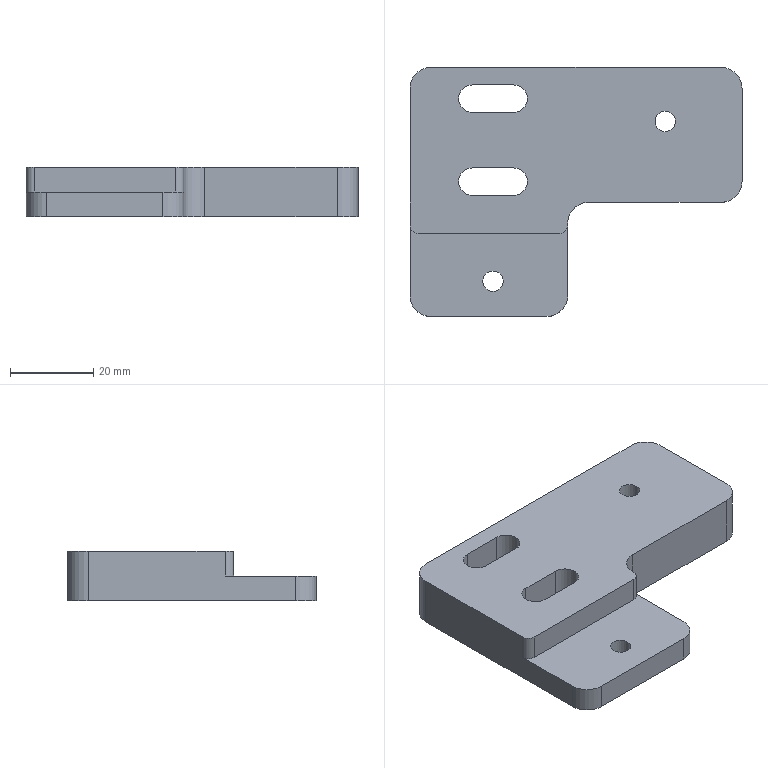Part | NX | 1 solid | 28 faces | box 80 x 60 x 12 mm | volume 36230 mm3 | cylinder 14 | plane 14 | commonest cylinder face diameters 10 x6 6.6 x4 4 x2 4.917 x2
STEP:
#1=CARTESIAN_POINT('',(-38.,-14.,6.));
#2=VERTEX_POINT('',#1);
#3=CARTESIAN_POINT('',(-40.,-12.,6.));
#4=VERTEX_POINT('',#3);
#5=CARTESIAN_POINT('',(-38.,-12.,6.));
#6=DIRECTION('',(0.,0.,-1.));
#7=DIRECTION('',(-0.7071,-0.7071,0.));
#8=AXIS2_PLACEMENT_3D('',#5,#6,#7);
#9=CIRCLE('',#8,2.);
#10=EDGE_CURVE('',#2,#4,#9,.T.);
#11=ORIENTED_EDGE('',*,*,#10,.T.);
#12=CARTESIAN_POINT('',(-40.,-12.,0.));
#13=VERTEX_POINT('',#12);
#14=CARTESIAN_POINT('',(-40.,-12.,0.));
#15=DIRECTION('',(0.,0.,-1.));
#16=VECTOR('',#15,1000.);
#17=LINE('',#14,#16);
#18=EDGE_CURVE('',#4,#13,#17,.T.);
#19=ORIENTED_EDGE('',*,*,#18,.T.);
#20=CARTESIAN_POINT('',(-38.,-14.,0.));
#21=VERTEX_POINT('',#20);
#22=CARTESIAN_POINT('',(-38.,-12.,0.));
#23=DIRECTION('',(0.,0.,1.));
#24=DIRECTION('',(-0.7071,-0.7071,0.));
#25=AXIS2_PLACEMENT_3D('',#22,#23,#24);
#26=CIRCLE('',#25,2.);
#27=EDGE_CURVE('',#13,#21,#26,.T.);
#28=ORIENTED_EDGE('',*,*,#27,.T.);
#29=CARTESIAN_POINT('',(-38.,-14.,0.));
#30=DIRECTION('',(0.,0.,1.));
#31=VECTOR('',#30,1000.);
#32=LINE('',#29,#31);
#33=EDGE_CURVE('',#21,#2,#32,.T.);
#34=ORIENTED_EDGE('',*,*,#33,.T.);
#35=EDGE_LOOP('',(#11,#19,#28,#34));
#36=FACE_BOUND('',#35,.T.);
#37=CARTESIAN_POINT('',(-38.,-12.,0.));
#38=DIRECTION('',(0.,0.,1.));
#39=DIRECTION('',(0.7071,0.7071,0.));
#40=AXIS2_PLACEMENT_3D('',#37,#38,#39);
#41=CYLINDRICAL_SURFACE('',#40,2.);
#42=ADVANCED_FACE('',(#36),#41,.T.);
#43=ORIENTED_EDGE('',*,*,#10,.F.);
#44=CARTESIAN_POINT('',(-4.,-14.,6.));
#45=VERTEX_POINT('',#44);
#46=CARTESIAN_POINT('',(-30.,-14.,6.));
#47=DIRECTION('',(1.,0.,0.));
#48=VECTOR('',#47,1000.);
#49=LINE('',#46,#48);
#50=EDGE_CURVE('',#2,#45,#49,.T.);
#51=ORIENTED_EDGE('',*,*,#50,.T.);
#52=CARTESIAN_POINT('',(-2.,-12.,6.));
#53=VERTEX_POINT('',#52);
#54=CARTESIAN_POINT('',(-4.,-12.,6.));
#55=DIRECTION('',(0.,0.,-1.));
#56=DIRECTION('',(0.7071,-0.7071,0.));
#57=AXIS2_PLACEMENT_3D('',#54,#55,#56);
#58=CIRCLE('',#57,2.);
#59=EDGE_CURVE('',#53,#45,#58,.T.);
#60=ORIENTED_EDGE('',*,*,#59,.F.);
#61=CARTESIAN_POINT('',(-2.,-11.5,6.));
#62=VERTEX_POINT('',#61);
#63=CARTESIAN_POINT('',(-2.,-8.875,6.));
#64=DIRECTION('',(0.,1.,0.));
#65=VECTOR('',#64,1000.);
#66=LINE('',#63,#65);
#67=EDGE_CURVE('',#53,#62,#66,.T.);
#68=ORIENTED_EDGE('',*,*,#67,.T.);
#69=CARTESIAN_POINT('',(3.,-6.5,6.));
#70=VERTEX_POINT('',#69);
#71=CARTESIAN_POINT('',(3.,-11.5,6.));
#72=DIRECTION('',(0.,0.,1.));
#73=DIRECTION('',(-0.7071,0.7071,0.));
#74=AXIS2_PLACEMENT_3D('',#71,#72,#73);
#75=CIRCLE('',#74,5.);
#76=EDGE_CURVE('',#70,#62,#75,.T.);
#77=ORIENTED_EDGE('',*,*,#76,.F.);
#78=CARTESIAN_POINT('',(35.,-6.5,6.));
#79=VERTEX_POINT('',#78);
#80=CARTESIAN_POINT('',(-11.,-6.5,6.));
#81=DIRECTION('',(1.,0.,0.));
#82=VECTOR('',#81,1000.);
#83=LINE('',#80,#82);
#84=EDGE_CURVE('',#70,#79,#83,.T.);
#85=ORIENTED_EDGE('',*,*,#84,.T.);
#86=CARTESIAN_POINT('',(40.,-1.5,6.));
#87=VERTEX_POINT('',#86);
#88=CARTESIAN_POINT('',(35.,-1.5,6.));
#89=DIRECTION('',(0.,0.,-1.));
#90=DIRECTION('',(0.7071,-0.7071,0.));
#91=AXIS2_PLACEMENT_3D('',#88,#89,#90);
#92=CIRCLE('',#91,5.);
#93=EDGE_CURVE('',#87,#79,#92,.T.);
#94=ORIENTED_EDGE('',*,*,#93,.F.);
#95=CARTESIAN_POINT('',(40.,21.,6.));
#96=VERTEX_POINT('',#95);
#97=CARTESIAN_POINT('',(40.,-35.5,6.));
#98=DIRECTION('',(0.,1.,0.));
#99=VECTOR('',#98,1000.);
#100=LINE('',#97,#99);
#101=EDGE_CURVE('',#87,#96,#100,.T.);
#102=ORIENTED_EDGE('',*,*,#101,.T.);
#103=CARTESIAN_POINT('',(35.,26.,6.));
#104=VERTEX_POINT('',#103);
#105=CARTESIAN_POINT('',(35.,21.,6.));
#106=DIRECTION('',(0.,0.,-1.));
#107=DIRECTION('',(0.7071,0.7071,0.));
#108=AXIS2_PLACEMENT_3D('',#105,#106,#107);
#109=CIRCLE('',#108,5.);
#110=EDGE_CURVE('',#104,#96,#109,.T.);
#111=ORIENTED_EDGE('',*,*,#110,.F.);
#112=CARTESIAN_POINT('',(-35.,26.,6.));
#113=VERTEX_POINT('',#112);
#114=CARTESIAN_POINT('',(40.,26.,6.));
#115=DIRECTION('',(-1.,0.,0.));
#116=VECTOR('',#115,1000.);
#117=LINE('',#114,#116);
#118=EDGE_CURVE('',#104,#113,#117,.T.);
#119=ORIENTED_EDGE('',*,*,#118,.T.);
#120=CARTESIAN_POINT('',(-40.,21.,6.));
#121=VERTEX_POINT('',#120);
#122=CARTESIAN_POINT('',(-35.,21.,6.));
#123=DIRECTION('',(0.,0.,-1.));
#124=DIRECTION('',(-0.7071,0.7071,0.));
#125=AXIS2_PLACEMENT_3D('',#122,#123,#124);
#126=CIRCLE('',#125,5.);
#127=EDGE_CURVE('',#121,#113,#126,.T.);
#128=ORIENTED_EDGE('',*,*,#127,.F.);
#129=CARTESIAN_POINT('',(-40.,35.5,6.));
#130=DIRECTION('',(0.,-1.,0.));
#131=VECTOR('',#130,1000.);
#132=LINE('',#129,#131);
#133=EDGE_CURVE('',#121,#4,#132,.T.);
#134=ORIENTED_EDGE('',*,*,#133,.T.);
#135=EDGE_LOOP('',(#43,#51,#60,#68,#77,#85,#94,#102,#111,#119,#128,#134));
#136=FACE_BOUND('',#135,.T.);
#137=CARTESIAN_POINT('',(-15.,1.8,6.));
#138=VERTEX_POINT('',#137);
#139=CARTESIAN_POINT('',(-15.,-4.8,6.));
#140=VERTEX_POINT('',#139);
#141=CARTESIAN_POINT('',(-15.,-1.5,6.));
#142=DIRECTION('',(0.,0.,-1.));
#143=DIRECTION('',(0.,-1.,0.));
#144=AXIS2_PLACEMENT_3D('',#141,#142,#143);
#145=CIRCLE('',#144,3.3);
#146=EDGE_CURVE('',#138,#140,#145,.T.);
#147=ORIENTED_EDGE('',*,*,#146,.T.);
#148=CARTESIAN_POINT('',(-25.,-4.8,6.));
#149=VERTEX_POINT('',#148);
#150=CARTESIAN_POINT('',(-17.5,-4.8,6.));
#151=DIRECTION('',(-1.,0.,0.));
#152=VECTOR('',#151,1000.);
#153=LINE('',#150,#152);
#154=EDGE_CURVE('',#140,#149,#153,.T.);
#155=ORIENTED_EDGE('',*,*,#154,.T.);
#156=CARTESIAN_POINT('',(-25.,1.8,6.));
#157=VERTEX_POINT('',#156);
#158=CARTESIAN_POINT('',(-25.,-1.5,6.));
#159=DIRECTION('',(0.,0.,-1.));
#160=DIRECTION('',(0.,1.,0.));
#161=AXIS2_PLACEMENT_3D('',#158,#159,#160);
#162=CIRCLE('',#161,3.3);
#163=EDGE_CURVE('',#149,#157,#162,.T.);
#164=ORIENTED_EDGE('',*,*,#163,.T.);
#165=CARTESIAN_POINT('',(-22.5,1.8,6.));
#166=DIRECTION('',(1.,0.,0.));
#167=VECTOR('',#166,1000.);
#168=LINE('',#165,#167);
#169=EDGE_CURVE('',#157,#138,#168,.T.);
#170=ORIENTED_EDGE('',*,*,#169,.T.);
#171=EDGE_LOOP('',(#147,#155,#164,#170));
#172=FACE_BOUND('',#171,.T.);
#173=CARTESIAN_POINT('',(-15.,21.8,6.));
#174=VERTEX_POINT('',#173);
#175=CARTESIAN_POINT('',(-15.,15.2,6.));
#176=VERTEX_POINT('',#175);
#177=CARTESIAN_POINT('',(-15.,18.5,6.));
#178=DIRECTION('',(0.,0.,-1.));
#179=DIRECTION('',(0.,-1.,0.));
#180=AXIS2_PLACEMENT_3D('',#177,#178,#179);
#181=CIRCLE('',#180,3.3);
#182=EDGE_CURVE('',#174,#176,#181,.T.);
#183=ORIENTED_EDGE('',*,*,#182,.T.);
#184=CARTESIAN_POINT('',(-25.,15.2,6.));
#185=VERTEX_POINT('',#184);
#186=CARTESIAN_POINT('',(-17.5,15.2,6.));
#187=DIRECTION('',(-1.,0.,0.));
#188=VECTOR('',#187,1000.);
#189=LINE('',#186,#188);
#190=EDGE_CURVE('',#176,#185,#189,.T.);
#191=ORIENTED_EDGE('',*,*,#190,.T.);
#192=CARTESIAN_POINT('',(-25.,21.8,6.));
#193=VERTEX_POINT('',#192);
#194=CARTESIAN_POINT('',(-25.,18.5,6.));
#195=DIRECTION('',(0.,0.,-1.));
#196=DIRECTION('',(0.,1.,0.));
#197=AXIS2_PLACEMENT_3D('',#194,#195,#196);
#198=CIRCLE('',#197,3.3);
#199=EDGE_CURVE('',#185,#193,#198,.T.);
#200=ORIENTED_EDGE('',*,*,#199,.T.);
#201=CARTESIAN_POINT('',(-22.5,21.8,6.));
#202=DIRECTION('',(1.,0.,0.));
#203=VECTOR('',#202,1000.);
#204=LINE('',#201,#203);
#205=EDGE_CURVE('',#193,#174,#204,.T.);
#206=ORIENTED_EDGE('',*,*,#205,.T.);
#207=EDGE_LOOP('',(#183,#191,#200,#206));
#208=FACE_BOUND('',#207,.T.);
#209=CARTESIAN_POINT('',(23.959,13.,6.));
#210=VERTEX_POINT('',#209);
#211=CARTESIAN_POINT('',(19.041,13.,6.));
#212=VERTEX_POINT('',#211);
#213=CARTESIAN_POINT('',(21.5,13.,6.));
#214=DIRECTION('',(0.,0.,-1.));
#215=DIRECTION('',(1.,0.,0.));
#216=AXIS2_PLACEMENT_3D('',#213,#214,#215);
#217=CIRCLE('',#216,2.458);
#218=EDGE_CURVE('',#210,#212,#217,.T.);
#219=ORIENTED_EDGE('',*,*,#218,.T.);
#220=CARTESIAN_POINT('',(21.5,13.,6.));
#221=DIRECTION('',(0.,0.,-1.));
#222=DIRECTION('',(1.,0.,0.));
#223=AXIS2_PLACEMENT_3D('',#220,#221,#222);
#224=CIRCLE('',#223,2.458);
#225=EDGE_CURVE('',#212,#210,#224,.T.);
#226=ORIENTED_EDGE('',*,*,#225,.T.);
#227=EDGE_LOOP('',(#219,#226));
#228=FACE_BOUND('',#227,.T.);
#229=CARTESIAN_POINT('',(-20.,17.75,6.));
#230=DIRECTION('',(0.,0.,1.));
#231=DIRECTION('',(-1.,0.,0.));
#232=AXIS2_PLACEMENT_3D('',#229,#230,#231);
#233=PLANE('',#232);
#234=ADVANCED_FACE('',(#136,#172,#208,#228),#233,.T.);
#235=ORIENTED_EDGE('',*,*,#33,.F.);
#236=CARTESIAN_POINT('',(-4.,-14.,0.));
#237=VERTEX_POINT('',#236);
#238=CARTESIAN_POINT('',(-40.,-14.,0.));
#239=DIRECTION('',(1.,0.,0.));
#240=VECTOR('',#239,1000.);
#241=LINE('',#238,#240);
#242=EDGE_CURVE('',#21,#237,#241,.T.);
#243=ORIENTED_EDGE('',*,*,#242,.T.);
#244=CARTESIAN_POINT('',(-4.,-14.,3.));
#245=DIRECTION('',(0.,0.,-1.));
#246=VECTOR('',#245,1000.);
#247=LINE('',#244,#246);
#248=EDGE_CURVE('',#45,#237,#247,.T.);
#249=ORIENTED_EDGE('',*,*,#248,.F.);
#250=ORIENTED_EDGE('',*,*,#50,.F.);
#251=EDGE_LOOP('',(#235,#243,#249,#250));
#252=FACE_BOUND('',#251,.T.);
#253=CARTESIAN_POINT('',(-40.,-14.,0.));
#254=DIRECTION('',(0.,1.,0.));
#255=DIRECTION('',(0.,0.,-1.));
#256=AXIS2_PLACEMENT_3D('',#253,#254,#255);
#257=PLANE('',#256);
#258=ADVANCED_FACE('',(#252),#257,.F.);
#259=ORIENTED_EDGE('',*,*,#59,.T.);
#260=ORIENTED_EDGE('',*,*,#248,.T.);
#261=CARTESIAN_POINT('',(-2.,-12.,0.));
#262=VERTEX_POINT('',#261);
#263=CARTESIAN_POINT('',(-4.,-12.,0.));
#264=DIRECTION('',(0.,0.,1.));
#265=DIRECTION('',(0.7071,-0.7071,0.));
#266=AXIS2_PLACEMENT_3D('',#263,#264,#265);
#267=CIRCLE('',#266,2.);
#268=EDGE_CURVE('',#237,#262,#267,.T.);
#269=ORIENTED_EDGE('',*,*,#268,.T.);
#270=CARTESIAN_POINT('',(-2.,-12.,3.));
#271=DIRECTION('',(0.,0.,1.));
#272=VECTOR('',#271,1000.);
#273=LINE('',#270,#272);
#274=EDGE_CURVE('',#262,#53,#273,.T.);
#275=ORIENTED_EDGE('',*,*,#274,.T.);
#276=EDGE_LOOP('',(#259,#260,#269,#275));
#277=FACE_BOUND('',#276,.T.);
#278=CARTESIAN_POINT('',(-4.,-12.,3.));
#279=DIRECTION('',(0.,0.,-1.));
#280=DIRECTION('',(-0.7071,0.7071,0.));
#281=AXIS2_PLACEMENT_3D('',#278,#279,#280);
#282=CYLINDRICAL_SURFACE('',#281,2.);
#283=ADVANCED_FACE('',(#277),#282,.T.);
#284=ORIENTED_EDGE('',*,*,#274,.F.);
#285=CARTESIAN_POINT('',(-2.,-29.,0.));
#286=VERTEX_POINT('',#285);
#287=CARTESIAN_POINT('',(-2.,-34.75,0.));
#288=DIRECTION('',(0.,-1.,0.));
#289=VECTOR('',#288,1000.);
#290=LINE('',#287,#289);
#291=EDGE_CURVE('',#262,#286,#290,.T.);
#292=ORIENTED_EDGE('',*,*,#291,.T.);
#293=CARTESIAN_POINT('',(-2.,-29.,-6.));
#294=VERTEX_POINT('',#293);
#295=CARTESIAN_POINT('',(-2.,-29.,3.));
#296=DIRECTION('',(0.,0.,1.));
#297=VECTOR('',#296,1000.);
#298=LINE('',#295,#297);
#299=EDGE_CURVE('',#294,#286,#298,.T.);
#300=ORIENTED_EDGE('',*,*,#299,.F.);
#301=CARTESIAN_POINT('',(-2.,-11.5,-6.));
#302=VERTEX_POINT('',#301);
#303=CARTESIAN_POINT('',(-2.,-8.875,-6.));
#304=DIRECTION('',(0.,-1.,0.));
#305=VECTOR('',#304,1000.);
#306=LINE('',#303,#305);
#307=EDGE_CURVE('',#302,#294,#306,.T.);
#308=ORIENTED_EDGE('',*,*,#307,.F.);
#309=CARTESIAN_POINT('',(-2.,-11.5,6.));
#310=DIRECTION('',(0.,0.,-1.));
#311=VECTOR('',#310,1000.);
#312=LINE('',#309,#311);
#313=EDGE_CURVE('',#62,#302,#312,.T.);
#314=ORIENTED_EDGE('',*,*,#313,.F.);
#315=ORIENTED_EDGE('',*,*,#67,.F.);
#316=EDGE_LOOP('',(#284,#292,#300,#308,#314,#315));
#317=FACE_BOUND('',#316,.T.);
#318=CARTESIAN_POINT('',(-2.,-35.5,6.));
#319=DIRECTION('',(-1.,0.,0.));
#320=DIRECTION('',(0.,-1.,0.));
#321=AXIS2_PLACEMENT_3D('',#318,#319,#320);
#322=PLANE('',#321);
#323=ADVANCED_FACE('',(#317),#322,.F.);
#324=ORIENTED_EDGE('',*,*,#291,.F.);
#325=ORIENTED_EDGE('',*,*,#268,.F.);
#326=ORIENTED_EDGE('',*,*,#242,.F.);
#327=ORIENTED_EDGE('',*,*,#27,.F.);
#328=CARTESIAN_POINT('',(-40.,-29.,0.));
#329=VERTEX_POINT('',#328);
#330=CARTESIAN_POINT('',(-40.,0.75,0.));
#331=DIRECTION('',(0.,1.,0.));
#332=VECTOR('',#331,1000.);
#333=LINE('',#330,#332);
#334=EDGE_CURVE('',#329,#13,#333,.T.);
#335=ORIENTED_EDGE('',*,*,#334,.F.);
#336=CARTESIAN_POINT('',(-35.,-34.,0.));
#337=VERTEX_POINT('',#336);
#338=CARTESIAN_POINT('',(-35.,-29.,0.));
#339=DIRECTION('',(0.,0.,-1.));
#340=DIRECTION('',(-0.7071,-0.7071,0.));
#341=AXIS2_PLACEMENT_3D('',#338,#339,#340);
#342=CIRCLE('',#341,5.);
#343=EDGE_CURVE('',#337,#329,#342,.T.);
#344=ORIENTED_EDGE('',*,*,#343,.F.);
#345=CARTESIAN_POINT('',(-7.,-34.,0.));
#346=VERTEX_POINT('',#345);
#347=CARTESIAN_POINT('',(-40.,-34.,0.));
#348=DIRECTION('',(-1.,0.,0.));
#349=VECTOR('',#348,1000.);
#350=LINE('',#347,#349);
#351=EDGE_CURVE('',#346,#337,#350,.T.);
#352=ORIENTED_EDGE('',*,*,#351,.F.);
#353=CARTESIAN_POINT('',(-7.,-29.,0.));
#354=DIRECTION('',(0.,0.,-1.));
#355=DIRECTION('',(0.7071,-0.7071,0.));
#356=AXIS2_PLACEMENT_3D('',#353,#354,#355);
#357=CIRCLE('',#356,5.);
#358=EDGE_CURVE('',#286,#346,#357,.T.);
#359=ORIENTED_EDGE('',*,*,#358,.F.);
#360=EDGE_LOOP('',(#324,#325,#326,#327,#335,#344,#352,#359));
#361=FACE_BOUND('',#360,.T.);
#362=CARTESIAN_POINT('',(-22.459,-25.5,0.));
#363=VERTEX_POINT('',#362);
#364=CARTESIAN_POINT('',(-20.,-25.5,0.));
#365=DIRECTION('',(0.,0.,1.));
#366=DIRECTION('',(1.,0.,0.));
#367=AXIS2_PLACEMENT_3D('',#364,#365,#366);
#368=CIRCLE('',#367,2.458);
#369=EDGE_CURVE('',#363,#363,#368,.T.);
#370=ORIENTED_EDGE('',*,*,#369,.F.);
#371=EDGE_LOOP('',(#370));
#372=FACE_BOUND('',#371,.T.);
#373=CARTESIAN_POINT('',(-40.,-34.,0.));
#374=DIRECTION('',(0.,0.,-1.));
#375=DIRECTION('',(0.,-1.,0.));
#376=AXIS2_PLACEMENT_3D('',#373,#374,#375);
#377=PLANE('',#376);
#378=ADVANCED_FACE('',(#361,#372),#377,.F.);
#379=ORIENTED_EDGE('',*,*,#358,.T.);
#380=CARTESIAN_POINT('',(-7.,-34.,-6.));
#381=VERTEX_POINT('',#380);
#382=CARTESIAN_POINT('',(-7.,-34.,3.));
#383=DIRECTION('',(0.,0.,-1.));
#384=VECTOR('',#383,1000.);
#385=LINE('',#382,#384);
#386=EDGE_CURVE('',#346,#381,#385,.T.);
#387=ORIENTED_EDGE('',*,*,#386,.T.);
#388=CARTESIAN_POINT('',(-7.,-29.,-6.));
#389=DIRECTION('',(0.,0.,1.));
#390=DIRECTION('',(0.7071,-0.7071,0.));
#391=AXIS2_PLACEMENT_3D('',#388,#389,#390);
#392=CIRCLE('',#391,5.);
#393=EDGE_CURVE('',#381,#294,#392,.T.);
#394=ORIENTED_EDGE('',*,*,#393,.T.);
#395=ORIENTED_EDGE('',*,*,#299,.T.);
#396=EDGE_LOOP('',(#379,#387,#394,#395));
#397=FACE_BOUND('',#396,.T.);
#398=CARTESIAN_POINT('',(-7.,-29.,3.));
#399=DIRECTION('',(0.,0.,1.));
#400=DIRECTION('',(-0.7071,0.7071,0.));
#401=AXIS2_PLACEMENT_3D('',#398,#399,#400);
#402=CYLINDRICAL_SURFACE('',#401,5.);
#403=ADVANCED_FACE('',(#397),#402,.T.);
#404=ORIENTED_EDGE('',*,*,#351,.T.);
#405=CARTESIAN_POINT('',(-35.,-34.,-6.));
#406=VERTEX_POINT('',#405);
#407=CARTESIAN_POINT('',(-35.,-34.,0.));
#408=DIRECTION('',(0.,0.,1.));
#409=VECTOR('',#408,1000.);
#410=LINE('',#407,#409);
#411=EDGE_CURVE('',#406,#337,#410,.T.);
#412=ORIENTED_EDGE('',*,*,#411,.F.);
#413=CARTESIAN_POINT('',(-40.,-34.,-6.));
#414=DIRECTION('',(-1.,0.,0.));
#415=VECTOR('',#414,1000.);
#416=LINE('',#413,#415);
#417=EDGE_CURVE('',#381,#406,#416,.T.);
#418=ORIENTED_EDGE('',*,*,#417,.F.);
#419=ORIENTED_EDGE('',*,*,#386,.F.);
#420=EDGE_LOOP('',(#404,#412,#418,#419));
#421=FACE_BOUND('',#420,.T.);
#422=CARTESIAN_POINT('',(-40.,-34.,0.));
#423=DIRECTION('',(0.,-1.,0.));
#424=DIRECTION('',(-1.,0.,0.));
#425=AXIS2_PLACEMENT_3D('',#422,#423,#424);
#426=PLANE('',#425);
#427=ADVANCED_FACE('',(#421),#426,.T.);
#428=ORIENTED_EDGE('',*,*,#393,.F.);
#429=ORIENTED_EDGE('',*,*,#417,.T.);
#430=CARTESIAN_POINT('',(-40.,-29.,-6.));
#431=VERTEX_POINT('',#430);
#432=CARTESIAN_POINT('',(-35.,-29.,-6.));
#433=DIRECTION('',(0.,0.,1.));
#434=DIRECTION('',(-0.7071,-0.7071,0.));
#435=AXIS2_PLACEMENT_3D('',#432,#433,#434);
#436=CIRCLE('',#435,5.);
#437=EDGE_CURVE('',#431,#406,#436,.T.);
#438=ORIENTED_EDGE('',*,*,#437,.F.);
#439=CARTESIAN_POINT('',(-40.,21.,-6.));
#440=VERTEX_POINT('',#439);
#441=CARTESIAN_POINT('',(-40.,35.5,-6.));
#442=DIRECTION('',(0.,1.,0.));
#443=VECTOR('',#442,1000.);
#444=LINE('',#441,#443);
#445=EDGE_CURVE('',#431,#440,#444,.T.);
#446=ORIENTED_EDGE('',*,*,#445,.T.);
#447=CARTESIAN_POINT('',(-35.,26.,-6.));
#448=VERTEX_POINT('',#447);
#449=CARTESIAN_POINT('',(-35.,21.,-6.));
#450=DIRECTION('',(0.,0.,1.));
#451=DIRECTION('',(-0.7071,0.7071,0.));
#452=AXIS2_PLACEMENT_3D('',#449,#450,#451);
#453=CIRCLE('',#452,5.);
#454=EDGE_CURVE('',#448,#440,#453,.T.);
#455=ORIENTED_EDGE('',*,*,#454,.F.);
#456=CARTESIAN_POINT('',(35.,26.,-6.));
#457=VERTEX_POINT('',#456);
#458=CARTESIAN_POINT('',(40.,26.,-6.));
#459=DIRECTION('',(1.,0.,0.));
#460=VECTOR('',#459,1000.);
#461=LINE('',#458,#460);
#462=EDGE_CURVE('',#448,#457,#461,.T.);
#463=ORIENTED_EDGE('',*,*,#462,.T.);
#464=CARTESIAN_POINT('',(40.,21.,-6.));
#465=VERTEX_POINT('',#464);
#466=CARTESIAN_POINT('',(35.,21.,-6.));
#467=DIRECTION('',(0.,0.,1.));
#468=DIRECTION('',(0.7071,0.7071,0.));
#469=AXIS2_PLACEMENT_3D('',#466,#467,#468);
#470=CIRCLE('',#469,5.);
#471=EDGE_CURVE('',#465,#457,#470,.T.);
#472=ORIENTED_EDGE('',*,*,#471,.F.);
#473=CARTESIAN_POINT('',(40.,-1.5,-6.));
#474=VERTEX_POINT('',#473);
#475=CARTESIAN_POINT('',(40.,-35.5,-6.));
#476=DIRECTION('',(0.,-1.,0.));
#477=VECTOR('',#476,1000.);
#478=LINE('',#475,#477);
#479=EDGE_CURVE('',#465,#474,#478,.T.);
#480=ORIENTED_EDGE('',*,*,#479,.T.);
#481=CARTESIAN_POINT('',(35.,-6.5,-6.));
#482=VERTEX_POINT('',#481);
#483=CARTESIAN_POINT('',(35.,-1.5,-6.));
#484=DIRECTION('',(0.,0.,1.));
#485=DIRECTION('',(0.7071,-0.7071,0.));
#486=AXIS2_PLACEMENT_3D('',#483,#484,#485);
#487=CIRCLE('',#486,5.);
#488=EDGE_CURVE('',#482,#474,#487,.T.);
#489=ORIENTED_EDGE('',*,*,#488,.F.);
#490=CARTESIAN_POINT('',(3.,-6.5,-6.));
#491=VERTEX_POINT('',#490);
#492=CARTESIAN_POINT('',(-11.,-6.5,-6.));
#493=DIRECTION('',(-1.,0.,0.));
#494=VECTOR('',#493,1000.);
#495=LINE('',#492,#494);
#496=EDGE_CURVE('',#482,#491,#495,.T.);
#497=ORIENTED_EDGE('',*,*,#496,.T.);
#498=CARTESIAN_POINT('',(3.,-11.5,-6.));
#499=DIRECTION('',(0.,0.,-1.));
#500=DIRECTION('',(-0.7071,0.7071,0.));
#501=AXIS2_PLACEMENT_3D('',#498,#499,#500);
#502=CIRCLE('',#501,5.);
#503=EDGE_CURVE('',#302,#491,#502,.T.);
#504=ORIENTED_EDGE('',*,*,#503,.F.);
#505=ORIENTED_EDGE('',*,*,#307,.T.);
#506=EDGE_LOOP('',(#428,#429,#438,#446,#455,#463,#472,#480,#489,#497,#504,#505));
#507=FACE_BOUND('',#506,.T.);
#508=CARTESIAN_POINT('',(19.041,13.,-6.));
#509=VERTEX_POINT('',#508);
#510=CARTESIAN_POINT('',(21.5,13.,-6.));
#511=DIRECTION('',(0.,0.,1.));
#512=DIRECTION('',(1.,0.,0.));
#513=AXIS2_PLACEMENT_3D('',#510,#511,#512);
#514=CIRCLE('',#513,2.458);
#515=EDGE_CURVE('',#509,#509,#514,.T.);
#516=ORIENTED_EDGE('',*,*,#515,.T.);
#517=EDGE_LOOP('',(#516));
#518=FACE_BOUND('',#517,.T.);
#519=CARTESIAN_POINT('',(-22.459,-25.5,-6.));
#520=VERTEX_POINT('',#519);
#521=CARTESIAN_POINT('',(-20.,-25.5,-6.));
#522=DIRECTION('',(0.,0.,1.));
#523=DIRECTION('',(1.,0.,0.));
#524=AXIS2_PLACEMENT_3D('',#521,#522,#523);
#525=CIRCLE('',#524,2.458);
#526=EDGE_CURVE('',#520,#520,#525,.T.);
#527=ORIENTED_EDGE('',*,*,#526,.T.);
#528=EDGE_LOOP('',(#527));
#529=FACE_BOUND('',#528,.T.);
#530=CARTESIAN_POINT('',(-15.,-4.8,-6.));
#531=VERTEX_POINT('',#530);
#532=CARTESIAN_POINT('',(-15.,1.8,-6.));
#533=VERTEX_POINT('',#532);
#534=CARTESIAN_POINT('',(-15.,-1.5,-6.));
#535=DIRECTION('',(0.,0.,1.));
#536=DIRECTION('',(0.,-1.,0.));
#537=AXIS2_PLACEMENT_3D('',#534,#535,#536);
#538=CIRCLE('',#537,3.3);
#539=EDGE_CURVE('',#531,#533,#538,.T.);
#540=ORIENTED_EDGE('',*,*,#539,.T.);
#541=CARTESIAN_POINT('',(-25.,1.8,-6.));
#542=VERTEX_POINT('',#541);
#543=CARTESIAN_POINT('',(-22.5,1.8,-6.));
#544=DIRECTION('',(-1.,0.,0.));
#545=VECTOR('',#544,1000.);
#546=LINE('',#543,#545);
#547=EDGE_CURVE('',#533,#542,#546,.T.);
#548=ORIENTED_EDGE('',*,*,#547,.T.);
#549=CARTESIAN_POINT('',(-25.,-4.8,-6.));
#550=VERTEX_POINT('',#549);
#551=CARTESIAN_POINT('',(-25.,-1.5,-6.));
#552=DIRECTION('',(0.,0.,1.));
#553=DIRECTION('',(0.,1.,0.));
#554=AXIS2_PLACEMENT_3D('',#551,#552,#553);
#555=CIRCLE('',#554,3.3);
#556=EDGE_CURVE('',#542,#550,#555,.T.);
#557=ORIENTED_EDGE('',*,*,#556,.T.);
#558=CARTESIAN_POINT('',(-17.5,-4.8,-6.));
#559=DIRECTION('',(1.,0.,0.));
#560=VECTOR('',#559,1000.);
#561=LINE('',#558,#560);
#562=EDGE_CURVE('',#550,#531,#561,.T.);
#563=ORIENTED_EDGE('',*,*,#562,.T.);
#564=EDGE_LOOP('',(#540,#548,#557,#563));
#565=FACE_BOUND('',#564,.T.);
#566=CARTESIAN_POINT('',(-15.,15.2,-6.));
#567=VERTEX_POINT('',#566);
#568=CARTESIAN_POINT('',(-15.,21.8,-6.));
#569=VERTEX_POINT('',#568);
#570=CARTESIAN_POINT('',(-15.,18.5,-6.));
#571=DIRECTION('',(0.,0.,1.));
#572=DIRECTION('',(0.,-1.,0.));
#573=AXIS2_PLACEMENT_3D('',#570,#571,#572);
#574=CIRCLE('',#573,3.3);
#575=EDGE_CURVE('',#567,#569,#574,.T.);
#576=ORIENTED_EDGE('',*,*,#575,.T.);
#577=CARTESIAN_POINT('',(-25.,21.8,-6.));
#578=VERTEX_POINT('',#577);
#579=CARTESIAN_POINT('',(-22.5,21.8,-6.));
#580=DIRECTION('',(-1.,0.,0.));
#581=VECTOR('',#580,1000.);
#582=LINE('',#579,#581);
#583=EDGE_CURVE('',#569,#578,#582,.T.);
#584=ORIENTED_EDGE('',*,*,#583,.T.);
#585=CARTESIAN_POINT('',(-25.,15.2,-6.));
#586=VERTEX_POINT('',#585);
#587=CARTESIAN_POINT('',(-25.,18.5,-6.));
#588=DIRECTION('',(0.,0.,1.));
#589=DIRECTION('',(0.,1.,0.));
#590=AXIS2_PLACEMENT_3D('',#587,#588,#589);
#591=CIRCLE('',#590,3.3);
#592=EDGE_CURVE('',#578,#586,#591,.T.);
#593=ORIENTED_EDGE('',*,*,#592,.T.);
#594=CARTESIAN_POINT('',(-17.5,15.2,-6.));
#595=DIRECTION('',(1.,0.,0.));
#596=VECTOR('',#595,1000.);
#597=LINE('',#594,#596);
#598=EDGE_CURVE('',#586,#567,#597,.T.);
#599=ORIENTED_EDGE('',*,*,#598,.T.);
#600=EDGE_LOOP('',(#576,#584,#593,#599));
#601=FACE_BOUND('',#600,.T.);
#602=CARTESIAN_POINT('',(-20.,17.75,-6.));
#603=DIRECTION('',(0.,0.,-1.));
#604=DIRECTION('',(1.,0.,0.));
#605=AXIS2_PLACEMENT_3D('',#602,#603,#604);
#606=PLANE('',#605);
#607=ADVANCED_FACE('',(#507,#518,#529,#565,#601),#606,.T.);
#608=ORIENTED_EDGE('',*,*,#343,.T.);
#609=CARTESIAN_POINT('',(-40.,-29.,0.));
#610=DIRECTION('',(0.,0.,-1.));
#611=VECTOR('',#610,1000.);
#612=LINE('',#609,#611);
#613=EDGE_CURVE('',#329,#431,#612,.T.);
#614=ORIENTED_EDGE('',*,*,#613,.T.);
#615=ORIENTED_EDGE('',*,*,#437,.T.);
#616=ORIENTED_EDGE('',*,*,#411,.T.);
#617=EDGE_LOOP('',(#608,#614,#615,#616));
#618=FACE_BOUND('',#617,.T.);
#619=CARTESIAN_POINT('',(-35.,-29.,0.));
#620=DIRECTION('',(0.,0.,1.));
#621=DIRECTION('',(0.7071,0.7071,0.));
#622=AXIS2_PLACEMENT_3D('',#619,#620,#621);
#623=CYLINDRICAL_SURFACE('',#622,5.);
#624=ADVANCED_FACE('',(#618),#623,.T.);
#625=ORIENTED_EDGE('',*,*,#18,.F.);
#626=ORIENTED_EDGE('',*,*,#133,.F.);
#627=CARTESIAN_POINT('',(-40.,21.,0.));
#628=DIRECTION('',(0.,0.,1.));
#629=VECTOR('',#628,1000.);
#630=LINE('',#627,#629);
#631=EDGE_CURVE('',#440,#121,#630,.T.);
#632=ORIENTED_EDGE('',*,*,#631,.F.);
#633=ORIENTED_EDGE('',*,*,#445,.F.);
#634=ORIENTED_EDGE('',*,*,#613,.F.);
#635=ORIENTED_EDGE('',*,*,#334,.T.);
#636=EDGE_LOOP('',(#625,#626,#632,#633,#634,#635));
#637=FACE_BOUND('',#636,.T.);
#638=CARTESIAN_POINT('',(-40.,35.5,0.));
#639=DIRECTION('',(-1.,0.,0.));
#640=DIRECTION('',(0.,1.,0.));
#641=AXIS2_PLACEMENT_3D('',#638,#639,#640);
#642=PLANE('',#641);
#643=ADVANCED_FACE('',(#637),#642,.T.);
#644=ORIENTED_EDGE('',*,*,#127,.T.);
#645=CARTESIAN_POINT('',(-35.,26.,0.));
#646=DIRECTION('',(0.,0.,-1.));
#647=VECTOR('',#646,1000.);
#648=LINE('',#645,#647);
#649=EDGE_CURVE('',#113,#448,#648,.T.);
#650=ORIENTED_EDGE('',*,*,#649,.T.);
#651=ORIENTED_EDGE('',*,*,#454,.T.);
#652=ORIENTED_EDGE('',*,*,#631,.T.);
#653=EDGE_LOOP('',(#644,#650,#651,#652));
#654=FACE_BOUND('',#653,.T.);
#655=CARTESIAN_POINT('',(-35.,21.,0.));
#656=DIRECTION('',(0.,0.,1.));
#657=DIRECTION('',(0.7071,-0.7071,0.));
#658=AXIS2_PLACEMENT_3D('',#655,#656,#657);
#659=CYLINDRICAL_SURFACE('',#658,5.);
#660=ADVANCED_FACE('',(#654),#659,.T.);
#661=ORIENTED_EDGE('',*,*,#649,.F.);
#662=ORIENTED_EDGE('',*,*,#118,.F.);
#663=CARTESIAN_POINT('',(35.,26.,0.));
#664=DIRECTION('',(0.,0.,1.));
#665=VECTOR('',#664,1000.);
#666=LINE('',#663,#665);
#667=EDGE_CURVE('',#457,#104,#666,.T.);
#668=ORIENTED_EDGE('',*,*,#667,.F.);
#669=ORIENTED_EDGE('',*,*,#462,.F.);
#670=EDGE_LOOP('',(#661,#662,#668,#669));
#671=FACE_BOUND('',#670,.T.);
#672=CARTESIAN_POINT('',(0.,26.,0.));
#673=DIRECTION('',(0.,1.,0.));
#674=DIRECTION('',(1.,0.,0.));
#675=AXIS2_PLACEMENT_3D('',#672,#673,#674);
#676=PLANE('',#675);
#677=ADVANCED_FACE('',(#671),#676,.T.);
#678=ORIENTED_EDGE('',*,*,#471,.T.);
#679=ORIENTED_EDGE('',*,*,#667,.T.);
#680=ORIENTED_EDGE('',*,*,#110,.T.);
#681=CARTESIAN_POINT('',(40.,21.,0.));
#682=DIRECTION('',(0.,0.,-1.));
#683=VECTOR('',#682,1000.);
#684=LINE('',#681,#683);
#685=EDGE_CURVE('',#96,#465,#684,.T.);
#686=ORIENTED_EDGE('',*,*,#685,.T.);
#687=EDGE_LOOP('',(#678,#679,#680,#686));
#688=FACE_BOUND('',#687,.T.);
#689=CARTESIAN_POINT('',(35.,21.,0.));
#690=DIRECTION('',(0.,0.,-1.));
#691=DIRECTION('',(-0.7071,-0.7071,0.));
#692=AXIS2_PLACEMENT_3D('',#689,#690,#691);
#693=CYLINDRICAL_SURFACE('',#692,5.);
#694=ADVANCED_FACE('',(#688),#693,.T.);
#695=ORIENTED_EDGE('',*,*,#685,.F.);
#696=ORIENTED_EDGE('',*,*,#101,.F.);
#697=CARTESIAN_POINT('',(40.,-1.5,3.));
#698=DIRECTION('',(0.,0.,1.));
#699=VECTOR('',#698,1000.);
#700=LINE('',#697,#699);
#701=EDGE_CURVE('',#474,#87,#700,.T.);
#702=ORIENTED_EDGE('',*,*,#701,.F.);
#703=ORIENTED_EDGE('',*,*,#479,.F.);
#704=EDGE_LOOP('',(#695,#696,#702,#703));
#705=FACE_BOUND('',#704,.T.);
#706=CARTESIAN_POINT('',(40.,-35.5,0.));
#707=DIRECTION('',(1.,0.,0.));
#708=DIRECTION('',(0.,-1.,0.));
#709=AXIS2_PLACEMENT_3D('',#706,#707,#708);
#710=PLANE('',#709);
#711=ADVANCED_FACE('',(#705),#710,.T.);
#712=ORIENTED_EDGE('',*,*,#218,.F.);
#713=ORIENTED_EDGE('',*,*,#225,.F.);
#714=CARTESIAN_POINT('',(19.041,13.,-2.55));
#715=DIRECTION('',(0.,0.,-1.));
#716=VECTOR('',#715,1000.);
#717=LINE('',#714,#716);
#718=EDGE_CURVE('',#212,#509,#717,.T.);
#719=ORIENTED_EDGE('',*,*,#718,.T.);
#720=ORIENTED_EDGE('',*,*,#515,.F.);
#721=ORIENTED_EDGE('',*,*,#718,.F.);
#722=EDGE_LOOP('',(#712,#713,#719,#720,#721));
#723=FACE_BOUND('',#722,.T.);
#724=CARTESIAN_POINT('',(21.5,13.,-2.55));
#725=DIRECTION('',(0.,0.,1.));
#726=DIRECTION('',(-1.,0.,0.));
#727=AXIS2_PLACEMENT_3D('',#724,#725,#726);
#728=CYLINDRICAL_SURFACE('',#727,2.458);
#729=ADVANCED_FACE('',(#723),#728,.F.);
#730=ORIENTED_EDGE('',*,*,#369,.T.);
#731=CARTESIAN_POINT('',(-22.459,-25.5,-2.55));
#732=DIRECTION('',(0.,0.,-1.));
#733=VECTOR('',#732,1000.);
#734=LINE('',#731,#733);
#735=EDGE_CURVE('',#363,#520,#734,.T.);
#736=ORIENTED_EDGE('',*,*,#735,.T.);
#737=ORIENTED_EDGE('',*,*,#526,.F.);
#738=ORIENTED_EDGE('',*,*,#735,.F.);
#739=EDGE_LOOP('',(#730,#736,#737,#738));
#740=FACE_BOUND('',#739,.T.);
#741=CARTESIAN_POINT('',(-20.,-25.5,-2.55));
#742=DIRECTION('',(0.,0.,1.));
#743=DIRECTION('',(-1.,0.,0.));
#744=AXIS2_PLACEMENT_3D('',#741,#742,#743);
#745=CYLINDRICAL_SURFACE('',#744,2.458);
#746=ADVANCED_FACE('',(#740),#745,.F.);
#747=ORIENTED_EDGE('',*,*,#76,.T.);
#748=ORIENTED_EDGE('',*,*,#313,.T.);
#749=ORIENTED_EDGE('',*,*,#503,.T.);
#750=CARTESIAN_POINT('',(3.,-6.5,6.));
#751=DIRECTION('',(0.,0.,1.));
#752=VECTOR('',#751,1000.);
#753=LINE('',#750,#752);
#754=EDGE_CURVE('',#491,#70,#753,.T.);
#755=ORIENTED_EDGE('',*,*,#754,.T.);
#756=EDGE_LOOP('',(#747,#748,#749,#755));
#757=FACE_BOUND('',#756,.T.);
#758=CARTESIAN_POINT('',(3.,-11.5,6.));
#759=DIRECTION('',(0.,0.,-1.));
#760=DIRECTION('',(0.7071,-0.7071,0.));
#761=AXIS2_PLACEMENT_3D('',#758,#759,#760);
#762=CYLINDRICAL_SURFACE('',#761,5.);
#763=ADVANCED_FACE('',(#757),#762,.F.);
#764=ORIENTED_EDGE('',*,*,#488,.T.);
#765=ORIENTED_EDGE('',*,*,#701,.T.);
#766=ORIENTED_EDGE('',*,*,#93,.T.);
#767=CARTESIAN_POINT('',(35.,-6.5,3.));
#768=DIRECTION('',(0.,0.,-1.));
#769=VECTOR('',#768,1000.);
#770=LINE('',#767,#769);
#771=EDGE_CURVE('',#79,#482,#770,.T.);
#772=ORIENTED_EDGE('',*,*,#771,.T.);
#773=EDGE_LOOP('',(#764,#765,#766,#772));
#774=FACE_BOUND('',#773,.T.);
#775=CARTESIAN_POINT('',(35.,-1.5,3.));
#776=DIRECTION('',(0.,0.,-1.));
#777=DIRECTION('',(-0.7071,0.7071,0.));
#778=AXIS2_PLACEMENT_3D('',#775,#776,#777);
#779=CYLINDRICAL_SURFACE('',#778,5.);
#780=ADVANCED_FACE('',(#774),#779,.T.);
#781=ORIENTED_EDGE('',*,*,#754,.F.);
#782=ORIENTED_EDGE('',*,*,#496,.F.);
#783=ORIENTED_EDGE('',*,*,#771,.F.);
#784=ORIENTED_EDGE('',*,*,#84,.F.);
#785=EDGE_LOOP('',(#781,#782,#783,#784));
#786=FACE_BOUND('',#785,.T.);
#787=CARTESIAN_POINT('',(-2.,-6.5,6.));
#788=DIRECTION('',(0.,1.,0.));
#789=DIRECTION('',(-1.,0.,0.));
#790=AXIS2_PLACEMENT_3D('',#787,#788,#789);
#791=PLANE('',#790);
#792=ADVANCED_FACE('',(#786),#791,.F.);
#793=ORIENTED_EDGE('',*,*,#592,.F.);
#794=CARTESIAN_POINT('',(-25.,21.8,6.));
#795=DIRECTION('',(0.,0.,-1.));
#796=VECTOR('',#795,1000.);
#797=LINE('',#794,#796);
#798=EDGE_CURVE('',#193,#578,#797,.T.);
#799=ORIENTED_EDGE('',*,*,#798,.F.);
#800=ORIENTED_EDGE('',*,*,#199,.F.);
#801=CARTESIAN_POINT('',(-25.,15.2,6.));
#802=DIRECTION('',(0.,0.,-1.));
#803=VECTOR('',#802,1000.);
#804=LINE('',#801,#803);
#805=EDGE_CURVE('',#185,#586,#804,.T.);
#806=ORIENTED_EDGE('',*,*,#805,.T.);
#807=EDGE_LOOP('',(#793,#799,#800,#806));
#808=FACE_BOUND('',#807,.T.);
#809=CARTESIAN_POINT('',(-25.,18.5,6.));
#810=DIRECTION('',(0.,0.,-1.));
#811=DIRECTION('',(0.,-1.,0.));
#812=AXIS2_PLACEMENT_3D('',#809,#810,#811);
#813=CYLINDRICAL_SURFACE('',#812,3.3);
#814=ADVANCED_FACE('',(#808),#813,.F.);
#815=ORIENTED_EDGE('',*,*,#598,.F.);
#816=ORIENTED_EDGE('',*,*,#805,.F.);
#817=ORIENTED_EDGE('',*,*,#190,.F.);
#818=CARTESIAN_POINT('',(-15.,15.2,6.));
#819=DIRECTION('',(0.,0.,-1.));
#820=VECTOR('',#819,1000.);
#821=LINE('',#818,#820);
#822=EDGE_CURVE('',#176,#567,#821,.T.);
#823=ORIENTED_EDGE('',*,*,#822,.T.);
#824=EDGE_LOOP('',(#815,#816,#817,#823));
#825=FACE_BOUND('',#824,.T.);
#826=CARTESIAN_POINT('',(-15.,15.2,6.));
#827=DIRECTION('',(0.,-1.,0.));
#828=DIRECTION('',(1.,0.,0.));
#829=AXIS2_PLACEMENT_3D('',#826,#827,#828);
#830=PLANE('',#829);
#831=ADVANCED_FACE('',(#825),#830,.F.);
#832=ORIENTED_EDGE('',*,*,#575,.F.);
#833=ORIENTED_EDGE('',*,*,#822,.F.);
#834=ORIENTED_EDGE('',*,*,#182,.F.);
#835=CARTESIAN_POINT('',(-15.,21.8,6.));
#836=DIRECTION('',(0.,0.,-1.));
#837=VECTOR('',#836,1000.);
#838=LINE('',#835,#837);
#839=EDGE_CURVE('',#174,#569,#838,.T.);
#840=ORIENTED_EDGE('',*,*,#839,.T.);
#841=EDGE_LOOP('',(#832,#833,#834,#840));
#842=FACE_BOUND('',#841,.T.);
#843=CARTESIAN_POINT('',(-15.,18.5,6.));
#844=DIRECTION('',(0.,0.,-1.));
#845=DIRECTION('',(0.,1.,0.));
#846=AXIS2_PLACEMENT_3D('',#843,#844,#845);
#847=CYLINDRICAL_SURFACE('',#846,3.3);
#848=ADVANCED_FACE('',(#842),#847,.F.);
#849=ORIENTED_EDGE('',*,*,#583,.F.);
#850=ORIENTED_EDGE('',*,*,#839,.F.);
#851=ORIENTED_EDGE('',*,*,#205,.F.);
#852=ORIENTED_EDGE('',*,*,#798,.T.);
#853=EDGE_LOOP('',(#849,#850,#851,#852));
#854=FACE_BOUND('',#853,.T.);
#855=CARTESIAN_POINT('',(-25.,21.8,6.));
#856=DIRECTION('',(0.,1.,0.));
#857=DIRECTION('',(-1.,0.,0.));
#858=AXIS2_PLACEMENT_3D('',#855,#856,#857);
#859=PLANE('',#858);
#860=ADVANCED_FACE('',(#854),#859,.F.);
#861=ORIENTED_EDGE('',*,*,#556,.F.);
#862=CARTESIAN_POINT('',(-25.,1.8,6.));
#863=DIRECTION('',(0.,0.,-1.));
#864=VECTOR('',#863,1000.);
#865=LINE('',#862,#864);
#866=EDGE_CURVE('',#157,#542,#865,.T.);
#867=ORIENTED_EDGE('',*,*,#866,.F.);
#868=ORIENTED_EDGE('',*,*,#163,.F.);
#869=CARTESIAN_POINT('',(-25.,-4.8,6.));
#870=DIRECTION('',(0.,0.,-1.));
#871=VECTOR('',#870,1000.);
#872=LINE('',#869,#871);
#873=EDGE_CURVE('',#149,#550,#872,.T.);
#874=ORIENTED_EDGE('',*,*,#873,.T.);
#875=EDGE_LOOP('',(#861,#867,#868,#874));
#876=FACE_BOUND('',#875,.T.);
#877=CARTESIAN_POINT('',(-25.,-1.5,6.));
#878=DIRECTION('',(0.,0.,-1.));
#879=DIRECTION('',(0.,-1.,0.));
#880=AXIS2_PLACEMENT_3D('',#877,#878,#879);
#881=CYLINDRICAL_SURFACE('',#880,3.3);
#882=ADVANCED_FACE('',(#876),#881,.F.);
#883=ORIENTED_EDGE('',*,*,#562,.F.);
#884=ORIENTED_EDGE('',*,*,#873,.F.);
#885=ORIENTED_EDGE('',*,*,#154,.F.);
#886=CARTESIAN_POINT('',(-15.,-4.8,6.));
#887=DIRECTION('',(0.,0.,-1.));
#888=VECTOR('',#887,1000.);
#889=LINE('',#886,#888);
#890=EDGE_CURVE('',#140,#531,#889,.T.);
#891=ORIENTED_EDGE('',*,*,#890,.T.);
#892=EDGE_LOOP('',(#883,#884,#885,#891));
#893=FACE_BOUND('',#892,.T.);
#894=CARTESIAN_POINT('',(-15.,-4.8,6.));
#895=DIRECTION('',(0.,-1.,0.));
#896=DIRECTION('',(1.,0.,0.));
#897=AXIS2_PLACEMENT_3D('',#894,#895,#896);
#898=PLANE('',#897);
#899=ADVANCED_FACE('',(#893),#898,.F.);
#900=ORIENTED_EDGE('',*,*,#539,.F.);
#901=ORIENTED_EDGE('',*,*,#890,.F.);
#902=ORIENTED_EDGE('',*,*,#146,.F.);
#903=CARTESIAN_POINT('',(-15.,1.8,6.));
#904=DIRECTION('',(0.,0.,-1.));
#905=VECTOR('',#904,1000.);
#906=LINE('',#903,#905);
#907=EDGE_CURVE('',#138,#533,#906,.T.);
#908=ORIENTED_EDGE('',*,*,#907,.T.);
#909=EDGE_LOOP('',(#900,#901,#902,#908));
#910=FACE_BOUND('',#909,.T.);
#911=CARTESIAN_POINT('',(-15.,-1.5,6.));
#912=DIRECTION('',(0.,0.,-1.));
#913=DIRECTION('',(0.,1.,0.));
#914=AXIS2_PLACEMENT_3D('',#911,#912,#913);
#915=CYLINDRICAL_SURFACE('',#914,3.3);
#916=ADVANCED_FACE('',(#910),#915,.F.);
#917=ORIENTED_EDGE('',*,*,#547,.F.);
#918=ORIENTED_EDGE('',*,*,#907,.F.);
#919=ORIENTED_EDGE('',*,*,#169,.F.);
#920=ORIENTED_EDGE('',*,*,#866,.T.);
#921=EDGE_LOOP('',(#917,#918,#919,#920));
#922=FACE_BOUND('',#921,.T.);
#923=CARTESIAN_POINT('',(-25.,1.8,6.));
#924=DIRECTION('',(0.,1.,0.));
#925=DIRECTION('',(-1.,0.,0.));
#926=AXIS2_PLACEMENT_3D('',#923,#924,#925);
#927=PLANE('',#926);
#928=ADVANCED_FACE('',(#922),#927,.F.);
#929=CLOSED_SHELL('',(#42,#234,#258,#283,#323,#378,#403,#427,#607,#624,#643,#660,#677,#694,#711,#729,#746,#763,#780,#792,#814,#831,#848,#860,#882,#899,#916,#928));
#930=MANIFOLD_SOLID_BREP('',#929);
#931=(LENGTH_UNIT()NAMED_UNIT(*)SI_UNIT(.MILLI.,.METRE.));
#932=UNCERTAINTY_MEASURE_WITH_UNIT(LENGTH_MEASURE(0.00001),#931,'','');
#933=(NAMED_UNIT(*)PLANE_ANGLE_UNIT()SI_UNIT($,.RADIAN.));
#934=(NAMED_UNIT(*)SI_UNIT($,.STERADIAN.)SOLID_ANGLE_UNIT());
#935=(GEOMETRIC_REPRESENTATION_CONTEXT(3)GLOBAL_UNCERTAINTY_ASSIGNED_CONTEXT((#932))GLOBAL_UNIT_ASSIGNED_CONTEXT((#931,#933,#934))REPRESENTATION_CONTEXT('',''));
#936=ADVANCED_BREP_SHAPE_REPRESENTATION('',(#930),#935);